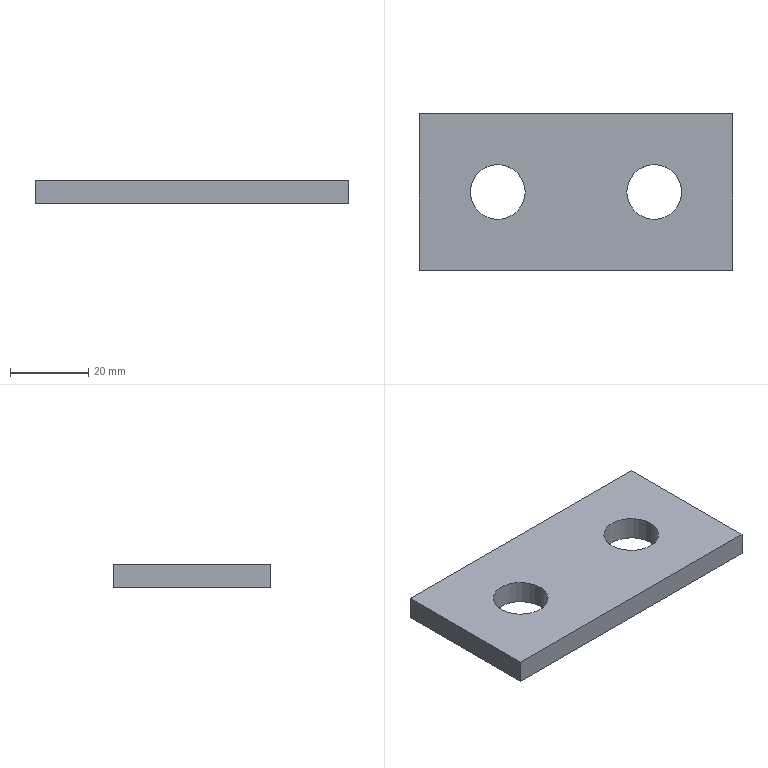Part | STEP file | 08-Baffle | 1 solid | 10 faces | box 80 x 40 x 6 mm | volume 17353 mm3 | plane 6 | cylinder 4 | commonest cylinder face diameters 14 x4
STEP:
#1=CARTESIAN_POINT('',(0.,0.,0.));
#2=DIRECTION('',(0.,0.,1.));
#3=DIRECTION('',(1.,0.,0.));
#4=AXIS2_PLACEMENT_3D('',#1,#2,#3);
#5=CARTESIAN_POINT('',(53.,-20.,6.));
#6=VERTEX_POINT('',#5);
#7=CARTESIAN_POINT('',(53.,-20.,0.));
#8=VERTEX_POINT('',#7);
#9=CARTESIAN_POINT('',(53.,-20.,6.));
#10=DIRECTION('',(0.,0.,-1.));
#11=VECTOR('',#10,1.);
#12=LINE('',#9,#11);
#13=CARTESIAN_POINT('',(60.,-20.,6.));
#14=DIRECTION('',(0.,0.,-1.));
#15=DIRECTION('',(-1.,0.,0.));
#16=AXIS2_PLACEMENT_3D('',#13,#14,#15);
#17=CYLINDRICAL_SURFACE('',#16,7.);
#18=CARTESIAN_POINT('',(6.283,0.));
#19=DIRECTION('',(0.,1.));
#20=VECTOR('',#19,1.);
#21=LINE('',#18,#20);
#22=(GEOMETRIC_REPRESENTATION_CONTEXT(2)PARAMETRIC_REPRESENTATION_CONTEXT()REPRESENTATION_CONTEXT('',''));
#23=DEFINITIONAL_REPRESENTATION('',(#21),#22);
#24=PCURVE('',#17,#23);
#25=CARTESIAN_POINT('',(60.,-20.,6.));
#26=DIRECTION('',(0.,0.,-1.));
#27=DIRECTION('',(-1.,0.,0.));
#28=AXIS2_PLACEMENT_3D('',#25,#26,#27);
#29=CYLINDRICAL_SURFACE('',#28,7.);
#30=CARTESIAN_POINT('',(0.,0.));
#31=DIRECTION('',(0.,1.));
#32=VECTOR('',#31,1.);
#33=LINE('',#30,#32);
#34=(GEOMETRIC_REPRESENTATION_CONTEXT(2)PARAMETRIC_REPRESENTATION_CONTEXT()REPRESENTATION_CONTEXT('',''));
#35=DEFINITIONAL_REPRESENTATION('',(#33),#34);
#36=PCURVE('',#29,#35);
#37=SURFACE_CURVE('',#12,(#24,#36),.PCURVE_S1.);
#38=EDGE_CURVE('',#6,#8,#37,.T.);
#39=ORIENTED_EDGE('',*,*,#38,.T.);
#40=CARTESIAN_POINT('',(67.,-20.,0.));
#41=VERTEX_POINT('',#40);
#42=CARTESIAN_POINT('',(60.,-20.,0.));
#43=DIRECTION('',(0.,0.,1.));
#44=DIRECTION('',(1.,0.,0.));
#45=AXIS2_PLACEMENT_3D('',#42,#43,#44);
#46=CIRCLE('',#45,7.);
#47=CARTESIAN_POINT('',(9.425,6.));
#48=DIRECTION('',(-1.,0.));
#49=VECTOR('',#48,1.);
#50=LINE('',#47,#49);
#51=(GEOMETRIC_REPRESENTATION_CONTEXT(2)PARAMETRIC_REPRESENTATION_CONTEXT()REPRESENTATION_CONTEXT('',''));
#52=DEFINITIONAL_REPRESENTATION('',(#50),#51);
#53=PCURVE('',#17,#52);
#54=CARTESIAN_POINT('',(0.,0.,0.));
#55=DIRECTION('',(0.,0.,1.));
#56=DIRECTION('',(1.,0.,0.));
#57=AXIS2_PLACEMENT_3D('',#54,#55,#56);
#58=PLANE('',#57);
#59=CARTESIAN_POINT('',(60.,-20.));
#60=DIRECTION('',(1.,0.));
#61=AXIS2_PLACEMENT_2D('',#59,#60);
#62=CIRCLE('',#61,7.);
#63=(GEOMETRIC_REPRESENTATION_CONTEXT(2)PARAMETRIC_REPRESENTATION_CONTEXT()REPRESENTATION_CONTEXT('',''));
#64=DEFINITIONAL_REPRESENTATION('',(#62),#63);
#65=PCURVE('',#58,#64);
#66=SURFACE_CURVE('',#46,(#53,#65),.PCURVE_S1.);
#67=EDGE_CURVE('',#8,#41,#66,.T.);
#68=ORIENTED_EDGE('',*,*,#67,.T.);
#69=CARTESIAN_POINT('',(67.,-20.,6.));
#70=VERTEX_POINT('',#69);
#71=CARTESIAN_POINT('',(67.,-20.,6.));
#72=DIRECTION('',(0.,0.,-1.));
#73=VECTOR('',#72,1.);
#74=LINE('',#71,#73);
#75=CARTESIAN_POINT('',(3.142,0.));
#76=DIRECTION('',(0.,1.));
#77=VECTOR('',#76,1.);
#78=LINE('',#75,#77);
#79=(GEOMETRIC_REPRESENTATION_CONTEXT(2)PARAMETRIC_REPRESENTATION_CONTEXT()REPRESENTATION_CONTEXT('',''));
#80=DEFINITIONAL_REPRESENTATION('',(#78),#79);
#81=PCURVE('',#17,#80);
#82=CARTESIAN_POINT('',(3.142,0.));
#83=DIRECTION('',(0.,1.));
#84=VECTOR('',#83,1.);
#85=LINE('',#82,#84);
#86=(GEOMETRIC_REPRESENTATION_CONTEXT(2)PARAMETRIC_REPRESENTATION_CONTEXT()REPRESENTATION_CONTEXT('',''));
#87=DEFINITIONAL_REPRESENTATION('',(#85),#86);
#88=PCURVE('',#29,#87);
#89=SURFACE_CURVE('',#74,(#81,#88),.PCURVE_S1.);
#90=EDGE_CURVE('',#70,#41,#89,.T.);
#91=ORIENTED_EDGE('',*,*,#90,.F.);
#92=CARTESIAN_POINT('',(60.,-20.,6.));
#93=DIRECTION('',(0.,0.,1.));
#94=DIRECTION('',(1.,0.,0.));
#95=AXIS2_PLACEMENT_3D('',#92,#93,#94);
#96=CIRCLE('',#95,7.);
#97=CARTESIAN_POINT('',(9.425,0.));
#98=DIRECTION('',(-1.,0.));
#99=VECTOR('',#98,1.);
#100=LINE('',#97,#99);
#101=(GEOMETRIC_REPRESENTATION_CONTEXT(2)PARAMETRIC_REPRESENTATION_CONTEXT()REPRESENTATION_CONTEXT('',''));
#102=DEFINITIONAL_REPRESENTATION('',(#100),#101);
#103=PCURVE('',#17,#102);
#104=CARTESIAN_POINT('',(0.,0.,6.));
#105=DIRECTION('',(0.,0.,1.));
#106=DIRECTION('',(1.,0.,0.));
#107=AXIS2_PLACEMENT_3D('',#104,#105,#106);
#108=PLANE('',#107);
#109=CARTESIAN_POINT('',(60.,-20.));
#110=DIRECTION('',(1.,0.));
#111=AXIS2_PLACEMENT_2D('',#109,#110);
#112=CIRCLE('',#111,7.);
#113=(GEOMETRIC_REPRESENTATION_CONTEXT(2)PARAMETRIC_REPRESENTATION_CONTEXT()REPRESENTATION_CONTEXT('',''));
#114=DEFINITIONAL_REPRESENTATION('',(#112),#113);
#115=PCURVE('',#108,#114);
#116=SURFACE_CURVE('',#96,(#103,#115),.PCURVE_S1.);
#117=EDGE_CURVE('',#6,#70,#116,.T.);
#118=ORIENTED_EDGE('',*,*,#117,.F.);
#119=EDGE_LOOP('',(#39,#68,#91,#118));
#120=FACE_BOUND('',#119,.F.);
#121=ADVANCED_FACE('',(#120),#17,.F.);
#122=CARTESIAN_POINT('',(13.,-20.,6.));
#123=VERTEX_POINT('',#122);
#124=CARTESIAN_POINT('',(13.,-20.,0.));
#125=VERTEX_POINT('',#124);
#126=CARTESIAN_POINT('',(13.,-20.,6.));
#127=DIRECTION('',(0.,0.,-1.));
#128=VECTOR('',#127,1.);
#129=LINE('',#126,#128);
#130=CARTESIAN_POINT('',(20.,-20.,6.));
#131=DIRECTION('',(0.,0.,-1.));
#132=DIRECTION('',(-1.,0.,0.));
#133=AXIS2_PLACEMENT_3D('',#130,#131,#132);
#134=CYLINDRICAL_SURFACE('',#133,7.);
#135=CARTESIAN_POINT('',(6.283,0.));
#136=DIRECTION('',(0.,1.));
#137=VECTOR('',#136,1.);
#138=LINE('',#135,#137);
#139=(GEOMETRIC_REPRESENTATION_CONTEXT(2)PARAMETRIC_REPRESENTATION_CONTEXT()REPRESENTATION_CONTEXT('',''));
#140=DEFINITIONAL_REPRESENTATION('',(#138),#139);
#141=PCURVE('',#134,#140);
#142=CARTESIAN_POINT('',(20.,-20.,6.));
#143=DIRECTION('',(0.,0.,-1.));
#144=DIRECTION('',(-1.,0.,0.));
#145=AXIS2_PLACEMENT_3D('',#142,#143,#144);
#146=CYLINDRICAL_SURFACE('',#145,7.);
#147=CARTESIAN_POINT('',(0.,0.));
#148=DIRECTION('',(0.,1.));
#149=VECTOR('',#148,1.);
#150=LINE('',#147,#149);
#151=(GEOMETRIC_REPRESENTATION_CONTEXT(2)PARAMETRIC_REPRESENTATION_CONTEXT()REPRESENTATION_CONTEXT('',''));
#152=DEFINITIONAL_REPRESENTATION('',(#150),#151);
#153=PCURVE('',#146,#152);
#154=SURFACE_CURVE('',#129,(#141,#153),.PCURVE_S1.);
#155=EDGE_CURVE('',#123,#125,#154,.T.);
#156=ORIENTED_EDGE('',*,*,#155,.T.);
#157=CARTESIAN_POINT('',(27.,-20.,0.));
#158=VERTEX_POINT('',#157);
#159=CARTESIAN_POINT('',(20.,-20.,0.));
#160=DIRECTION('',(0.,0.,1.));
#161=DIRECTION('',(1.,0.,0.));
#162=AXIS2_PLACEMENT_3D('',#159,#160,#161);
#163=CIRCLE('',#162,7.);
#164=CARTESIAN_POINT('',(9.425,6.));
#165=DIRECTION('',(-1.,0.));
#166=VECTOR('',#165,1.);
#167=LINE('',#164,#166);
#168=(GEOMETRIC_REPRESENTATION_CONTEXT(2)PARAMETRIC_REPRESENTATION_CONTEXT()REPRESENTATION_CONTEXT('',''));
#169=DEFINITIONAL_REPRESENTATION('',(#167),#168);
#170=PCURVE('',#134,#169);
#171=CARTESIAN_POINT('',(20.,-20.));
#172=DIRECTION('',(1.,0.));
#173=AXIS2_PLACEMENT_2D('',#171,#172);
#174=CIRCLE('',#173,7.);
#175=(GEOMETRIC_REPRESENTATION_CONTEXT(2)PARAMETRIC_REPRESENTATION_CONTEXT()REPRESENTATION_CONTEXT('',''));
#176=DEFINITIONAL_REPRESENTATION('',(#174),#175);
#177=PCURVE('',#58,#176);
#178=SURFACE_CURVE('',#163,(#170,#177),.PCURVE_S1.);
#179=EDGE_CURVE('',#125,#158,#178,.T.);
#180=ORIENTED_EDGE('',*,*,#179,.T.);
#181=CARTESIAN_POINT('',(27.,-20.,6.));
#182=VERTEX_POINT('',#181);
#183=CARTESIAN_POINT('',(27.,-20.,6.));
#184=DIRECTION('',(0.,0.,-1.));
#185=VECTOR('',#184,1.);
#186=LINE('',#183,#185);
#187=CARTESIAN_POINT('',(3.142,0.));
#188=DIRECTION('',(0.,1.));
#189=VECTOR('',#188,1.);
#190=LINE('',#187,#189);
#191=(GEOMETRIC_REPRESENTATION_CONTEXT(2)PARAMETRIC_REPRESENTATION_CONTEXT()REPRESENTATION_CONTEXT('',''));
#192=DEFINITIONAL_REPRESENTATION('',(#190),#191);
#193=PCURVE('',#134,#192);
#194=CARTESIAN_POINT('',(3.142,0.));
#195=DIRECTION('',(0.,1.));
#196=VECTOR('',#195,1.);
#197=LINE('',#194,#196);
#198=(GEOMETRIC_REPRESENTATION_CONTEXT(2)PARAMETRIC_REPRESENTATION_CONTEXT()REPRESENTATION_CONTEXT('',''));
#199=DEFINITIONAL_REPRESENTATION('',(#197),#198);
#200=PCURVE('',#146,#199);
#201=SURFACE_CURVE('',#186,(#193,#200),.PCURVE_S1.);
#202=EDGE_CURVE('',#182,#158,#201,.T.);
#203=ORIENTED_EDGE('',*,*,#202,.F.);
#204=CARTESIAN_POINT('',(20.,-20.,6.));
#205=DIRECTION('',(0.,0.,1.));
#206=DIRECTION('',(1.,0.,0.));
#207=AXIS2_PLACEMENT_3D('',#204,#205,#206);
#208=CIRCLE('',#207,7.);
#209=CARTESIAN_POINT('',(9.425,0.));
#210=DIRECTION('',(-1.,0.));
#211=VECTOR('',#210,1.);
#212=LINE('',#209,#211);
#213=(GEOMETRIC_REPRESENTATION_CONTEXT(2)PARAMETRIC_REPRESENTATION_CONTEXT()REPRESENTATION_CONTEXT('',''));
#214=DEFINITIONAL_REPRESENTATION('',(#212),#213);
#215=PCURVE('',#134,#214);
#216=CARTESIAN_POINT('',(20.,-20.));
#217=DIRECTION('',(1.,0.));
#218=AXIS2_PLACEMENT_2D('',#216,#217);
#219=CIRCLE('',#218,7.);
#220=(GEOMETRIC_REPRESENTATION_CONTEXT(2)PARAMETRIC_REPRESENTATION_CONTEXT()REPRESENTATION_CONTEXT('',''));
#221=DEFINITIONAL_REPRESENTATION('',(#219),#220);
#222=PCURVE('',#108,#221);
#223=SURFACE_CURVE('',#208,(#215,#222),.PCURVE_S1.);
#224=EDGE_CURVE('',#123,#182,#223,.T.);
#225=ORIENTED_EDGE('',*,*,#224,.F.);
#226=EDGE_LOOP('',(#156,#180,#203,#225));
#227=FACE_BOUND('',#226,.F.);
#228=ADVANCED_FACE('',(#227),#134,.F.);
#229=ORIENTED_EDGE('',*,*,#224,.F.);
#230=CARTESIAN_POINT('',(20.,-20.,6.));
#231=DIRECTION('',(0.,0.,1.));
#232=DIRECTION('',(1.,0.,0.));
#233=AXIS2_PLACEMENT_3D('',#230,#231,#232);
#234=CIRCLE('',#233,7.);
#235=CARTESIAN_POINT('',(20.,-20.));
#236=DIRECTION('',(1.,0.));
#237=AXIS2_PLACEMENT_2D('',#235,#236);
#238=CIRCLE('',#237,7.);
#239=(GEOMETRIC_REPRESENTATION_CONTEXT(2)PARAMETRIC_REPRESENTATION_CONTEXT()REPRESENTATION_CONTEXT('',''));
#240=DEFINITIONAL_REPRESENTATION('',(#238),#239);
#241=PCURVE('',#108,#240);
#242=CARTESIAN_POINT('',(3.142,0.));
#243=DIRECTION('',(-1.,0.));
#244=VECTOR('',#243,1.);
#245=LINE('',#242,#244);
#246=(GEOMETRIC_REPRESENTATION_CONTEXT(2)PARAMETRIC_REPRESENTATION_CONTEXT()REPRESENTATION_CONTEXT('',''));
#247=DEFINITIONAL_REPRESENTATION('',(#245),#246);
#248=PCURVE('',#146,#247);
#249=SURFACE_CURVE('',#234,(#241,#248),.PCURVE_S1.);
#250=EDGE_CURVE('',#182,#123,#249,.T.);
#251=ORIENTED_EDGE('',*,*,#250,.F.);
#252=EDGE_LOOP('',(#229,#251));
#253=FACE_BOUND('',#252,.T.);
#254=CARTESIAN_POINT('',(0.,0.,6.));
#255=VERTEX_POINT('',#254);
#256=CARTESIAN_POINT('',(0.,-40.,6.));
#257=VERTEX_POINT('',#256);
#258=CARTESIAN_POINT('',(0.,0.,6.));
#259=DIRECTION('',(0.,-1.,0.));
#260=VECTOR('',#259,1.);
#261=LINE('',#258,#260);
#262=CARTESIAN_POINT('',(0.,0.));
#263=DIRECTION('',(0.,-1.));
#264=VECTOR('',#263,1.);
#265=LINE('',#262,#264);
#266=(GEOMETRIC_REPRESENTATION_CONTEXT(2)PARAMETRIC_REPRESENTATION_CONTEXT()REPRESENTATION_CONTEXT('',''));
#267=DEFINITIONAL_REPRESENTATION('',(#265),#266);
#268=PCURVE('',#108,#267);
#269=CARTESIAN_POINT('',(0.,0.,6.));
#270=DIRECTION('',(1.,0.,0.));
#271=DIRECTION('',(0.,1.,0.));
#272=AXIS2_PLACEMENT_3D('',#269,#270,#271);
#273=PLANE('',#272);
#274=CARTESIAN_POINT('',(0.,0.));
#275=DIRECTION('',(-1.,0.));
#276=VECTOR('',#275,1.);
#277=LINE('',#274,#276);
#278=(GEOMETRIC_REPRESENTATION_CONTEXT(2)PARAMETRIC_REPRESENTATION_CONTEXT()REPRESENTATION_CONTEXT('',''));
#279=DEFINITIONAL_REPRESENTATION('',(#277),#278);
#280=PCURVE('',#273,#279);
#281=SURFACE_CURVE('',#261,(#268,#280),.PCURVE_S1.);
#282=EDGE_CURVE('',#255,#257,#281,.T.);
#283=ORIENTED_EDGE('',*,*,#282,.T.);
#284=CARTESIAN_POINT('',(80.,-40.,6.));
#285=VERTEX_POINT('',#284);
#286=CARTESIAN_POINT('',(0.,-40.,6.));
#287=DIRECTION('',(1.,0.,0.));
#288=VECTOR('',#287,1.);
#289=LINE('',#286,#288);
#290=CARTESIAN_POINT('',(0.,-40.));
#291=DIRECTION('',(1.,0.));
#292=VECTOR('',#291,1.);
#293=LINE('',#290,#292);
#294=(GEOMETRIC_REPRESENTATION_CONTEXT(2)PARAMETRIC_REPRESENTATION_CONTEXT()REPRESENTATION_CONTEXT('',''));
#295=DEFINITIONAL_REPRESENTATION('',(#293),#294);
#296=PCURVE('',#108,#295);
#297=CARTESIAN_POINT('',(0.,-40.,6.));
#298=DIRECTION('',(0.,1.,0.));
#299=DIRECTION('',(0.,0.,1.));
#300=AXIS2_PLACEMENT_3D('',#297,#298,#299);
#301=PLANE('',#300);
#302=CARTESIAN_POINT('',(0.,0.));
#303=DIRECTION('',(0.,1.));
#304=VECTOR('',#303,1.);
#305=LINE('',#302,#304);
#306=(GEOMETRIC_REPRESENTATION_CONTEXT(2)PARAMETRIC_REPRESENTATION_CONTEXT()REPRESENTATION_CONTEXT('',''));
#307=DEFINITIONAL_REPRESENTATION('',(#305),#306);
#308=PCURVE('',#301,#307);
#309=SURFACE_CURVE('',#289,(#296,#308),.PCURVE_S1.);
#310=EDGE_CURVE('',#257,#285,#309,.T.);
#311=ORIENTED_EDGE('',*,*,#310,.T.);
#312=CARTESIAN_POINT('',(80.,0.,6.));
#313=VERTEX_POINT('',#312);
#314=CARTESIAN_POINT('',(80.,0.,6.));
#315=DIRECTION('',(0.,1.,0.));
#316=VECTOR('',#315,1.);
#317=LINE('',#314,#316);
#318=CARTESIAN_POINT('',(80.,0.));
#319=DIRECTION('',(0.,1.));
#320=VECTOR('',#319,1.);
#321=LINE('',#318,#320);
#322=(GEOMETRIC_REPRESENTATION_CONTEXT(2)PARAMETRIC_REPRESENTATION_CONTEXT()REPRESENTATION_CONTEXT('',''));
#323=DEFINITIONAL_REPRESENTATION('',(#321),#322);
#324=PCURVE('',#108,#323);
#325=CARTESIAN_POINT('',(80.,0.,6.));
#326=DIRECTION('',(-1.,0.,0.));
#327=DIRECTION('',(0.,0.,1.));
#328=AXIS2_PLACEMENT_3D('',#325,#326,#327);
#329=PLANE('',#328);
#330=CARTESIAN_POINT('',(0.,0.));
#331=DIRECTION('',(0.,1.));
#332=VECTOR('',#331,1.);
#333=LINE('',#330,#332);
#334=(GEOMETRIC_REPRESENTATION_CONTEXT(2)PARAMETRIC_REPRESENTATION_CONTEXT()REPRESENTATION_CONTEXT('',''));
#335=DEFINITIONAL_REPRESENTATION('',(#333),#334);
#336=PCURVE('',#329,#335);
#337=SURFACE_CURVE('',#317,(#324,#336),.PCURVE_S1.);
#338=EDGE_CURVE('',#285,#313,#337,.T.);
#339=ORIENTED_EDGE('',*,*,#338,.T.);
#340=CARTESIAN_POINT('',(0.,0.,6.));
#341=DIRECTION('',(-1.,0.,0.));
#342=VECTOR('',#341,1.);
#343=LINE('',#340,#342);
#344=CARTESIAN_POINT('',(0.,0.));
#345=DIRECTION('',(-1.,0.));
#346=VECTOR('',#345,1.);
#347=LINE('',#344,#346);
#348=(GEOMETRIC_REPRESENTATION_CONTEXT(2)PARAMETRIC_REPRESENTATION_CONTEXT()REPRESENTATION_CONTEXT('',''));
#349=DEFINITIONAL_REPRESENTATION('',(#347),#348);
#350=PCURVE('',#108,#349);
#351=CARTESIAN_POINT('',(0.,0.,6.));
#352=DIRECTION('',(0.,-1.,0.));
#353=DIRECTION('',(0.,0.,-1.));
#354=AXIS2_PLACEMENT_3D('',#351,#352,#353);
#355=PLANE('',#354);
#356=CARTESIAN_POINT('',(0.,0.));
#357=DIRECTION('',(0.,-1.));
#358=VECTOR('',#357,1.);
#359=LINE('',#356,#358);
#360=(GEOMETRIC_REPRESENTATION_CONTEXT(2)PARAMETRIC_REPRESENTATION_CONTEXT()REPRESENTATION_CONTEXT('',''));
#361=DEFINITIONAL_REPRESENTATION('',(#359),#360);
#362=PCURVE('',#355,#361);
#363=SURFACE_CURVE('',#343,(#350,#362),.PCURVE_S1.);
#364=EDGE_CURVE('',#313,#255,#363,.T.);
#365=ORIENTED_EDGE('',*,*,#364,.T.);
#366=EDGE_LOOP('',(#283,#311,#339,#365));
#367=FACE_BOUND('',#366,.T.);
#368=ORIENTED_EDGE('',*,*,#117,.F.);
#369=CARTESIAN_POINT('',(60.,-20.,6.));
#370=DIRECTION('',(0.,0.,1.));
#371=DIRECTION('',(1.,0.,0.));
#372=AXIS2_PLACEMENT_3D('',#369,#370,#371);
#373=CIRCLE('',#372,7.);
#374=CARTESIAN_POINT('',(60.,-20.));
#375=DIRECTION('',(1.,0.));
#376=AXIS2_PLACEMENT_2D('',#374,#375);
#377=CIRCLE('',#376,7.);
#378=(GEOMETRIC_REPRESENTATION_CONTEXT(2)PARAMETRIC_REPRESENTATION_CONTEXT()REPRESENTATION_CONTEXT('',''));
#379=DEFINITIONAL_REPRESENTATION('',(#377),#378);
#380=PCURVE('',#108,#379);
#381=CARTESIAN_POINT('',(3.142,0.));
#382=DIRECTION('',(-1.,0.));
#383=VECTOR('',#382,1.);
#384=LINE('',#381,#383);
#385=(GEOMETRIC_REPRESENTATION_CONTEXT(2)PARAMETRIC_REPRESENTATION_CONTEXT()REPRESENTATION_CONTEXT('',''));
#386=DEFINITIONAL_REPRESENTATION('',(#384),#385);
#387=PCURVE('',#29,#386);
#388=SURFACE_CURVE('',#373,(#380,#387),.PCURVE_S1.);
#389=EDGE_CURVE('',#70,#6,#388,.T.);
#390=ORIENTED_EDGE('',*,*,#389,.F.);
#391=EDGE_LOOP('',(#368,#390));
#392=FACE_BOUND('',#391,.T.);
#393=ADVANCED_FACE('',(#253,#367,#392),#108,.T.);
#394=ORIENTED_EDGE('',*,*,#179,.T.);
#395=CARTESIAN_POINT('',(20.,-20.,0.));
#396=DIRECTION('',(0.,0.,1.));
#397=DIRECTION('',(1.,0.,0.));
#398=AXIS2_PLACEMENT_3D('',#395,#396,#397);
#399=CIRCLE('',#398,7.);
#400=CARTESIAN_POINT('',(20.,-20.));
#401=DIRECTION('',(1.,0.));
#402=AXIS2_PLACEMENT_2D('',#400,#401);
#403=CIRCLE('',#402,7.);
#404=(GEOMETRIC_REPRESENTATION_CONTEXT(2)PARAMETRIC_REPRESENTATION_CONTEXT()REPRESENTATION_CONTEXT('',''));
#405=DEFINITIONAL_REPRESENTATION('',(#403),#404);
#406=PCURVE('',#58,#405);
#407=CARTESIAN_POINT('',(3.142,6.));
#408=DIRECTION('',(-1.,0.));
#409=VECTOR('',#408,1.);
#410=LINE('',#407,#409);
#411=(GEOMETRIC_REPRESENTATION_CONTEXT(2)PARAMETRIC_REPRESENTATION_CONTEXT()REPRESENTATION_CONTEXT('',''));
#412=DEFINITIONAL_REPRESENTATION('',(#410),#411);
#413=PCURVE('',#146,#412);
#414=SURFACE_CURVE('',#399,(#406,#413),.PCURVE_S1.);
#415=EDGE_CURVE('',#158,#125,#414,.T.);
#416=ORIENTED_EDGE('',*,*,#415,.T.);
#417=EDGE_LOOP('',(#394,#416));
#418=FACE_BOUND('',#417,.T.);
#419=CARTESIAN_POINT('',(0.,0.,0.));
#420=VERTEX_POINT('',#419);
#421=CARTESIAN_POINT('',(0.,-40.,0.));
#422=VERTEX_POINT('',#421);
#423=CARTESIAN_POINT('',(0.,0.,0.));
#424=DIRECTION('',(0.,-1.,0.));
#425=VECTOR('',#424,1.);
#426=LINE('',#423,#425);
#427=CARTESIAN_POINT('',(0.,0.));
#428=DIRECTION('',(0.,-1.));
#429=VECTOR('',#428,1.);
#430=LINE('',#427,#429);
#431=(GEOMETRIC_REPRESENTATION_CONTEXT(2)PARAMETRIC_REPRESENTATION_CONTEXT()REPRESENTATION_CONTEXT('',''));
#432=DEFINITIONAL_REPRESENTATION('',(#430),#431);
#433=PCURVE('',#58,#432);
#434=CARTESIAN_POINT('',(0.,-6.));
#435=DIRECTION('',(-1.,0.));
#436=VECTOR('',#435,1.);
#437=LINE('',#434,#436);
#438=(GEOMETRIC_REPRESENTATION_CONTEXT(2)PARAMETRIC_REPRESENTATION_CONTEXT()REPRESENTATION_CONTEXT('',''));
#439=DEFINITIONAL_REPRESENTATION('',(#437),#438);
#440=PCURVE('',#273,#439);
#441=SURFACE_CURVE('',#426,(#433,#440),.PCURVE_S1.);
#442=EDGE_CURVE('',#420,#422,#441,.T.);
#443=ORIENTED_EDGE('',*,*,#442,.F.);
#444=CARTESIAN_POINT('',(80.,0.,0.));
#445=VERTEX_POINT('',#444);
#446=CARTESIAN_POINT('',(0.,0.,0.));
#447=DIRECTION('',(-1.,0.,0.));
#448=VECTOR('',#447,1.);
#449=LINE('',#446,#448);
#450=CARTESIAN_POINT('',(0.,0.));
#451=DIRECTION('',(-1.,0.));
#452=VECTOR('',#451,1.);
#453=LINE('',#450,#452);
#454=(GEOMETRIC_REPRESENTATION_CONTEXT(2)PARAMETRIC_REPRESENTATION_CONTEXT()REPRESENTATION_CONTEXT('',''));
#455=DEFINITIONAL_REPRESENTATION('',(#453),#454);
#456=PCURVE('',#58,#455);
#457=CARTESIAN_POINT('',(6.,0.));
#458=DIRECTION('',(0.,-1.));
#459=VECTOR('',#458,1.);
#460=LINE('',#457,#459);
#461=(GEOMETRIC_REPRESENTATION_CONTEXT(2)PARAMETRIC_REPRESENTATION_CONTEXT()REPRESENTATION_CONTEXT('',''));
#462=DEFINITIONAL_REPRESENTATION('',(#460),#461);
#463=PCURVE('',#355,#462);
#464=SURFACE_CURVE('',#449,(#456,#463),.PCURVE_S1.);
#465=EDGE_CURVE('',#445,#420,#464,.T.);
#466=ORIENTED_EDGE('',*,*,#465,.F.);
#467=CARTESIAN_POINT('',(80.,-40.,0.));
#468=VERTEX_POINT('',#467);
#469=CARTESIAN_POINT('',(80.,0.,0.));
#470=DIRECTION('',(0.,1.,0.));
#471=VECTOR('',#470,1.);
#472=LINE('',#469,#471);
#473=CARTESIAN_POINT('',(80.,0.));
#474=DIRECTION('',(0.,1.));
#475=VECTOR('',#474,1.);
#476=LINE('',#473,#475);
#477=(GEOMETRIC_REPRESENTATION_CONTEXT(2)PARAMETRIC_REPRESENTATION_CONTEXT()REPRESENTATION_CONTEXT('',''));
#478=DEFINITIONAL_REPRESENTATION('',(#476),#477);
#479=PCURVE('',#58,#478);
#480=CARTESIAN_POINT('',(-6.,0.));
#481=DIRECTION('',(0.,1.));
#482=VECTOR('',#481,1.);
#483=LINE('',#480,#482);
#484=(GEOMETRIC_REPRESENTATION_CONTEXT(2)PARAMETRIC_REPRESENTATION_CONTEXT()REPRESENTATION_CONTEXT('',''));
#485=DEFINITIONAL_REPRESENTATION('',(#483),#484);
#486=PCURVE('',#329,#485);
#487=SURFACE_CURVE('',#472,(#479,#486),.PCURVE_S1.);
#488=EDGE_CURVE('',#468,#445,#487,.T.);
#489=ORIENTED_EDGE('',*,*,#488,.F.);
#490=CARTESIAN_POINT('',(0.,-40.,0.));
#491=DIRECTION('',(1.,0.,0.));
#492=VECTOR('',#491,1.);
#493=LINE('',#490,#492);
#494=CARTESIAN_POINT('',(0.,-40.));
#495=DIRECTION('',(1.,0.));
#496=VECTOR('',#495,1.);
#497=LINE('',#494,#496);
#498=(GEOMETRIC_REPRESENTATION_CONTEXT(2)PARAMETRIC_REPRESENTATION_CONTEXT()REPRESENTATION_CONTEXT('',''));
#499=DEFINITIONAL_REPRESENTATION('',(#497),#498);
#500=PCURVE('',#58,#499);
#501=CARTESIAN_POINT('',(-6.,0.));
#502=DIRECTION('',(0.,1.));
#503=VECTOR('',#502,1.);
#504=LINE('',#501,#503);
#505=(GEOMETRIC_REPRESENTATION_CONTEXT(2)PARAMETRIC_REPRESENTATION_CONTEXT()REPRESENTATION_CONTEXT('',''));
#506=DEFINITIONAL_REPRESENTATION('',(#504),#505);
#507=PCURVE('',#301,#506);
#508=SURFACE_CURVE('',#493,(#500,#507),.PCURVE_S1.);
#509=EDGE_CURVE('',#422,#468,#508,.T.);
#510=ORIENTED_EDGE('',*,*,#509,.F.);
#511=EDGE_LOOP('',(#443,#466,#489,#510));
#512=FACE_BOUND('',#511,.T.);
#513=ORIENTED_EDGE('',*,*,#67,.T.);
#514=CARTESIAN_POINT('',(60.,-20.,0.));
#515=DIRECTION('',(0.,0.,1.));
#516=DIRECTION('',(1.,0.,0.));
#517=AXIS2_PLACEMENT_3D('',#514,#515,#516);
#518=CIRCLE('',#517,7.);
#519=CARTESIAN_POINT('',(60.,-20.));
#520=DIRECTION('',(1.,0.));
#521=AXIS2_PLACEMENT_2D('',#519,#520);
#522=CIRCLE('',#521,7.);
#523=(GEOMETRIC_REPRESENTATION_CONTEXT(2)PARAMETRIC_REPRESENTATION_CONTEXT()REPRESENTATION_CONTEXT('',''));
#524=DEFINITIONAL_REPRESENTATION('',(#522),#523);
#525=PCURVE('',#58,#524);
#526=CARTESIAN_POINT('',(3.142,6.));
#527=DIRECTION('',(-1.,0.));
#528=VECTOR('',#527,1.);
#529=LINE('',#526,#528);
#530=(GEOMETRIC_REPRESENTATION_CONTEXT(2)PARAMETRIC_REPRESENTATION_CONTEXT()REPRESENTATION_CONTEXT('',''));
#531=DEFINITIONAL_REPRESENTATION('',(#529),#530);
#532=PCURVE('',#29,#531);
#533=SURFACE_CURVE('',#518,(#525,#532),.PCURVE_S1.);
#534=EDGE_CURVE('',#41,#8,#533,.T.);
#535=ORIENTED_EDGE('',*,*,#534,.T.);
#536=EDGE_LOOP('',(#513,#535));
#537=FACE_BOUND('',#536,.T.);
#538=ADVANCED_FACE('',(#418,#512,#537),#58,.F.);
#539=ORIENTED_EDGE('',*,*,#442,.T.);
#540=CARTESIAN_POINT('',(0.,-40.,6.));
#541=DIRECTION('',(0.,0.,-1.));
#542=VECTOR('',#541,1.);
#543=LINE('',#540,#542);
#544=CARTESIAN_POINT('',(-40.,0.));
#545=DIRECTION('',(0.,-1.));
#546=VECTOR('',#545,1.);
#547=LINE('',#544,#546);
#548=(GEOMETRIC_REPRESENTATION_CONTEXT(2)PARAMETRIC_REPRESENTATION_CONTEXT()REPRESENTATION_CONTEXT('',''));
#549=DEFINITIONAL_REPRESENTATION('',(#547),#548);
#550=PCURVE('',#273,#549);
#551=CARTESIAN_POINT('',(0.,0.));
#552=DIRECTION('',(-1.,0.));
#553=VECTOR('',#552,1.);
#554=LINE('',#551,#553);
#555=(GEOMETRIC_REPRESENTATION_CONTEXT(2)PARAMETRIC_REPRESENTATION_CONTEXT()REPRESENTATION_CONTEXT('',''));
#556=DEFINITIONAL_REPRESENTATION('',(#554),#555);
#557=PCURVE('',#301,#556);
#558=SURFACE_CURVE('',#543,(#550,#557),.PCURVE_S1.);
#559=EDGE_CURVE('',#257,#422,#558,.T.);
#560=ORIENTED_EDGE('',*,*,#559,.F.);
#561=ORIENTED_EDGE('',*,*,#282,.F.);
#562=CARTESIAN_POINT('',(0.,0.,6.));
#563=DIRECTION('',(0.,0.,-1.));
#564=VECTOR('',#563,1.);
#565=LINE('',#562,#564);
#566=CARTESIAN_POINT('',(0.,0.));
#567=DIRECTION('',(0.,-1.));
#568=VECTOR('',#567,1.);
#569=LINE('',#566,#568);
#570=(GEOMETRIC_REPRESENTATION_CONTEXT(2)PARAMETRIC_REPRESENTATION_CONTEXT()REPRESENTATION_CONTEXT('',''));
#571=DEFINITIONAL_REPRESENTATION('',(#569),#570);
#572=PCURVE('',#273,#571);
#573=CARTESIAN_POINT('',(0.,0.));
#574=DIRECTION('',(1.,0.));
#575=VECTOR('',#574,1.);
#576=LINE('',#573,#575);
#577=(GEOMETRIC_REPRESENTATION_CONTEXT(2)PARAMETRIC_REPRESENTATION_CONTEXT()REPRESENTATION_CONTEXT('',''));
#578=DEFINITIONAL_REPRESENTATION('',(#576),#577);
#579=PCURVE('',#355,#578);
#580=SURFACE_CURVE('',#565,(#572,#579),.PCURVE_S1.);
#581=EDGE_CURVE('',#255,#420,#580,.T.);
#582=ORIENTED_EDGE('',*,*,#581,.T.);
#583=EDGE_LOOP('',(#539,#560,#561,#582));
#584=FACE_BOUND('',#583,.T.);
#585=ADVANCED_FACE('',(#584),#273,.F.);
#586=ORIENTED_EDGE('',*,*,#509,.T.);
#587=CARTESIAN_POINT('',(80.,-40.,6.));
#588=DIRECTION('',(0.,0.,-1.));
#589=VECTOR('',#588,1.);
#590=LINE('',#587,#589);
#591=CARTESIAN_POINT('',(0.,80.));
#592=DIRECTION('',(-1.,0.));
#593=VECTOR('',#592,1.);
#594=LINE('',#591,#593);
#595=(GEOMETRIC_REPRESENTATION_CONTEXT(2)PARAMETRIC_REPRESENTATION_CONTEXT()REPRESENTATION_CONTEXT('',''));
#596=DEFINITIONAL_REPRESENTATION('',(#594),#595);
#597=PCURVE('',#301,#596);
#598=CARTESIAN_POINT('',(0.,-40.));
#599=DIRECTION('',(-1.,0.));
#600=VECTOR('',#599,1.);
#601=LINE('',#598,#600);
#602=(GEOMETRIC_REPRESENTATION_CONTEXT(2)PARAMETRIC_REPRESENTATION_CONTEXT()REPRESENTATION_CONTEXT('',''));
#603=DEFINITIONAL_REPRESENTATION('',(#601),#602);
#604=PCURVE('',#329,#603);
#605=SURFACE_CURVE('',#590,(#597,#604),.PCURVE_S1.);
#606=EDGE_CURVE('',#285,#468,#605,.T.);
#607=ORIENTED_EDGE('',*,*,#606,.F.);
#608=ORIENTED_EDGE('',*,*,#310,.F.);
#609=ORIENTED_EDGE('',*,*,#559,.T.);
#610=EDGE_LOOP('',(#586,#607,#608,#609));
#611=FACE_BOUND('',#610,.T.);
#612=ADVANCED_FACE('',(#611),#301,.F.);
#613=ORIENTED_EDGE('',*,*,#488,.T.);
#614=CARTESIAN_POINT('',(80.,0.,6.));
#615=DIRECTION('',(0.,0.,-1.));
#616=VECTOR('',#615,1.);
#617=LINE('',#614,#616);
#618=CARTESIAN_POINT('',(0.,0.));
#619=DIRECTION('',(-1.,0.));
#620=VECTOR('',#619,1.);
#621=LINE('',#618,#620);
#622=(GEOMETRIC_REPRESENTATION_CONTEXT(2)PARAMETRIC_REPRESENTATION_CONTEXT()REPRESENTATION_CONTEXT('',''));
#623=DEFINITIONAL_REPRESENTATION('',(#621),#622);
#624=PCURVE('',#329,#623);
#625=CARTESIAN_POINT('',(0.,80.));
#626=DIRECTION('',(1.,0.));
#627=VECTOR('',#626,1.);
#628=LINE('',#625,#627);
#629=(GEOMETRIC_REPRESENTATION_CONTEXT(2)PARAMETRIC_REPRESENTATION_CONTEXT()REPRESENTATION_CONTEXT('',''));
#630=DEFINITIONAL_REPRESENTATION('',(#628),#629);
#631=PCURVE('',#355,#630);
#632=SURFACE_CURVE('',#617,(#624,#631),.PCURVE_S1.);
#633=EDGE_CURVE('',#313,#445,#632,.T.);
#634=ORIENTED_EDGE('',*,*,#633,.F.);
#635=ORIENTED_EDGE('',*,*,#338,.F.);
#636=ORIENTED_EDGE('',*,*,#606,.T.);
#637=EDGE_LOOP('',(#613,#634,#635,#636));
#638=FACE_BOUND('',#637,.T.);
#639=ADVANCED_FACE('',(#638),#329,.F.);
#640=ORIENTED_EDGE('',*,*,#465,.T.);
#641=ORIENTED_EDGE('',*,*,#581,.F.);
#642=ORIENTED_EDGE('',*,*,#364,.F.);
#643=ORIENTED_EDGE('',*,*,#633,.T.);
#644=EDGE_LOOP('',(#640,#641,#642,#643));
#645=FACE_BOUND('',#644,.T.);
#646=ADVANCED_FACE('',(#645),#355,.F.);
#647=ORIENTED_EDGE('',*,*,#415,.T.);
#648=ORIENTED_EDGE('',*,*,#155,.F.);
#649=ORIENTED_EDGE('',*,*,#250,.F.);
#650=ORIENTED_EDGE('',*,*,#202,.T.);
#651=EDGE_LOOP('',(#647,#648,#649,#650));
#652=FACE_BOUND('',#651,.F.);
#653=ADVANCED_FACE('',(#652),#146,.F.);
#654=ORIENTED_EDGE('',*,*,#534,.T.);
#655=ORIENTED_EDGE('',*,*,#38,.F.);
#656=ORIENTED_EDGE('',*,*,#389,.F.);
#657=ORIENTED_EDGE('',*,*,#90,.T.);
#658=EDGE_LOOP('',(#654,#655,#656,#657));
#659=FACE_BOUND('',#658,.F.);
#660=ADVANCED_FACE('',(#659),#29,.F.);
#661=CLOSED_SHELL('',(#121,#228,#393,#538,#585,#612,#639,#646,#653,#660));
#662=MANIFOLD_SOLID_BREP('',#661);
#663=(LENGTH_UNIT()NAMED_UNIT(*)SI_UNIT(.MILLI.,.METRE.));
#664=UNCERTAINTY_MEASURE_WITH_UNIT(LENGTH_MEASURE(0.0000001),#663,'','');
#665=(NAMED_UNIT(*)PLANE_ANGLE_UNIT()SI_UNIT($,.RADIAN.));
#666=(NAMED_UNIT(*)SI_UNIT($,.STERADIAN.)SOLID_ANGLE_UNIT());
#667=(GEOMETRIC_REPRESENTATION_CONTEXT(3)GLOBAL_UNCERTAINTY_ASSIGNED_CONTEXT((#664))GLOBAL_UNIT_ASSIGNED_CONTEXT((#663,#665,#666))REPRESENTATION_CONTEXT('',''));
#668=ADVANCED_BREP_SHAPE_REPRESENTATION('',(#4,#662),#667);